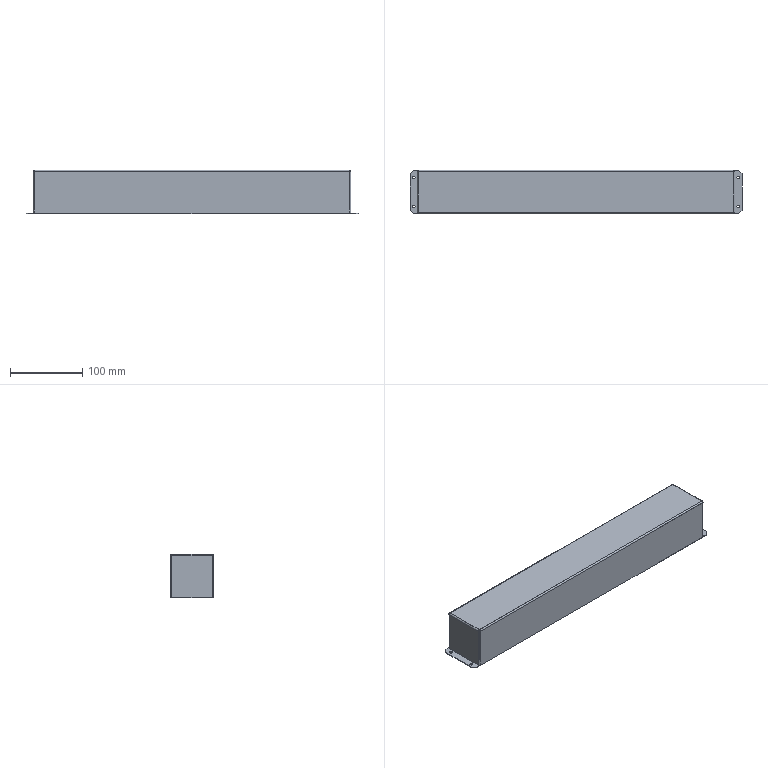Part | STEP file | CA-10-018Cylinder Cover_Default | 1 solid | 56 faces | box 458 x 60 x 60 mm | volume 82593 mm3 | cylinder 24 | plane 24 | sphere 8 | commonest cylinder face diameters 4 x16 2 x8